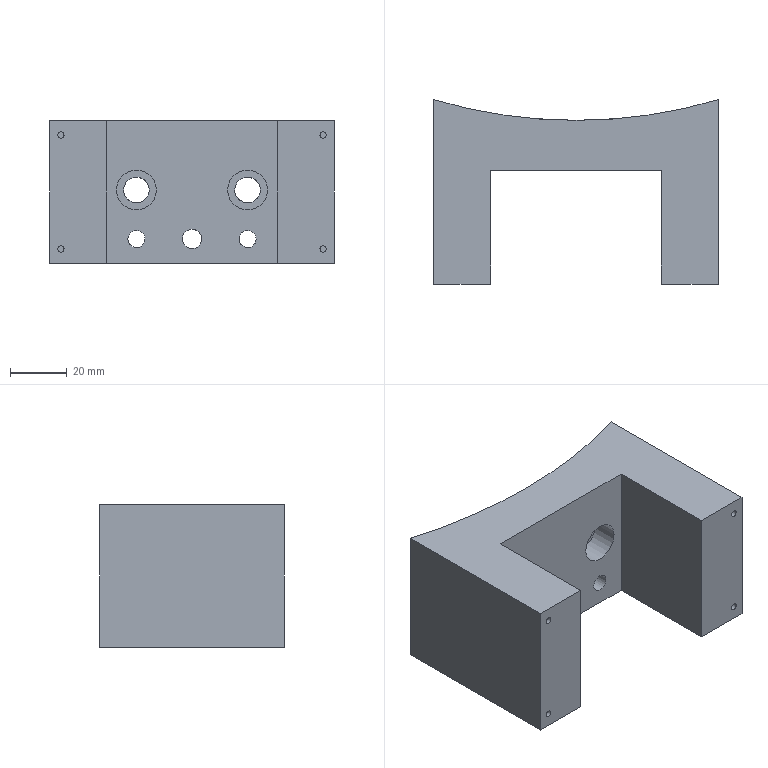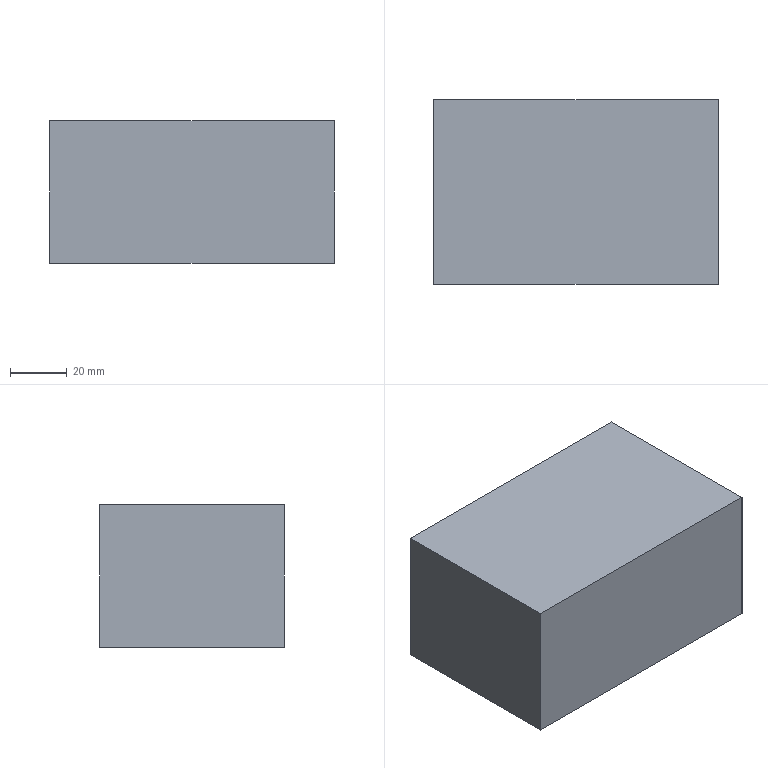CAM job | NX | 3+2 milling, drilling | part box 100 x 64.77 x 50 mm | stock box 100 x 64.77 x 50 mm
Tools:
number,name,description,diameter,corner_radius,flute_length,length,flutes
2,D50R0.8,Milling Tool-5 Parameters,50.0,0.8,50.0,75.0,2
3,ZXZ,Milling Tool-5 Parameters,6.0,0.0,50.0,75.0,2
9,9.0ZT,Drilling Tool,9.0,0.0,35.0,50.0,2
12,2.2ZT,Drilling Tool,2.2,0.0,35.0,50.0,2
16,6.8ZT,Drilling Tool,6.8,0.0,35.0,50.0,2
15,5.8ZT,Drilling Tool,5.8,0.0,35.0,50.0,2
13,6.0JD,Milling Tool-5 Parameters,6.0,0.0,30.0,30.0,4
14,14.0UZ,Milling Tool-5 Parameters,14.0,0.0,30.0,30.0,4
11,D10JING,Milling Tool-5 Parameters,10.0,0.0,50.0,75.0,2
7,D6A45,Milling Tool-5 Parameters,6.0,0.0,3.0,3.0,2
Operations:
program,operation,operation_type,tool,method,geometry_group,spindle_rpm,surface_speed,feed_per_tooth,feed_cut,feed_plunge,cut_length_mm,path_length_mm,cut_time_min,machine_time_min
1,ZLEVEL_PROFILE_1,ZLevelMilling,D50R0.8,METHOD,A,1200.0,188.0,0.625,1500.0,100.0,19146.255,19231.603,12.764,12.773
1,DRILLING,Operation,ZXZ,METHOD,A,3000.0,56.0,0.0417,250.0,0.0,36.0,414.109,0.144,0.1818
1,DRILLING_COPY,Operation,2.2ZT,METHOD,A,2000.0,13.0,0.025,100.0,0.0,56.0,353.274,0.56,0.5897
1,DRILLING_COPY_COPY,Operation,6.8ZT,METHOD,A,2000.0,42.0,0.045,180.0,0.0,24.073,188.145,0.1337,0.1501
1,DRILLING_COPY_COPY_COPY,Operation,5.8ZT,METHOD,A,2000.0,42.0,0.045,180.0,0.0,50.375,282.865,0.2799,0.3031
1,DRILLING_COPY_COPY_COPY_COPY,Operation,6.0JD,METHOD,A,1000.0,18.0,0.0125,50.0,0.0,44.89,271.896,0.8978,0.9205
1,DRILLING_COPY_1,Operation,9.0ZT,METHOD,A,1000.0,28.0,0.1,200.0,0.0,52.699,287.513,0.2635,0.287
1,DRILLING_COPY_1_COPY,Operation,14.0UZ,METHOD,A,1000.0,43.0,0.0375,150.0,0.0,24.0,230.115,0.16,0.1806
1,11,ZLevelMilling,D10JING,METHOD,A,5500.0,172.0,0.0909,1000.0,1000.0,394.769,925.635,0.3948,0.4479
1,FLOOR_WALL_1,VolumeBased25DMillingOperation,D10JING,METHOD,A,5000.0,157.0,0.1,1000.0,100.0,852.988,1357.096,0.853,0.9034
1,ZLEVEL_PROFILE_1_COPY_1_COPY,ZLevelMilling,D6A45,METHOD,A,7500.0,141.0,0.0667,1000.0,100.0,307.553,545.784,0.3076,0.3314
1,DRILLING_COPY_2,Operation,D6A45,METHOD,A,3000.0,56.0,0.0417,250.0,0.0,17.0,275.274,0.068,0.0938
2,ZLEVEL_PROFILE_1_COPY,ZLevelMilling,D50R0.8,METHOD,B,1200.0,188.0,0.625,1500.0,100.0,17082.963,17244.963,11.389,11.405
2,11_COPY,ZLevelMilling,D10JING,METHOD,B,5500.0,172.0,0.0909,1000.0,1000.0,457.214,909.124,0.4572,0.5024
2,ZLEVEL_PROFILE_1_COPY_1_COPY_COPY_COPY,ZLevelMilling,D6A45,METHOD,B,7500.0,141.0,0.0667,1000.0,100.0,420.786,480.786,0.4208,0.4268
3,ZLEVEL_PROFILE_1_COPY_1_COPY_COPY_COPY_COPY,ZLevelMilling,D6A45,METHOD,C,7500.0,141.0,0.0667,1000.0,100.0,420.786,480.786,0.4208,0.4268